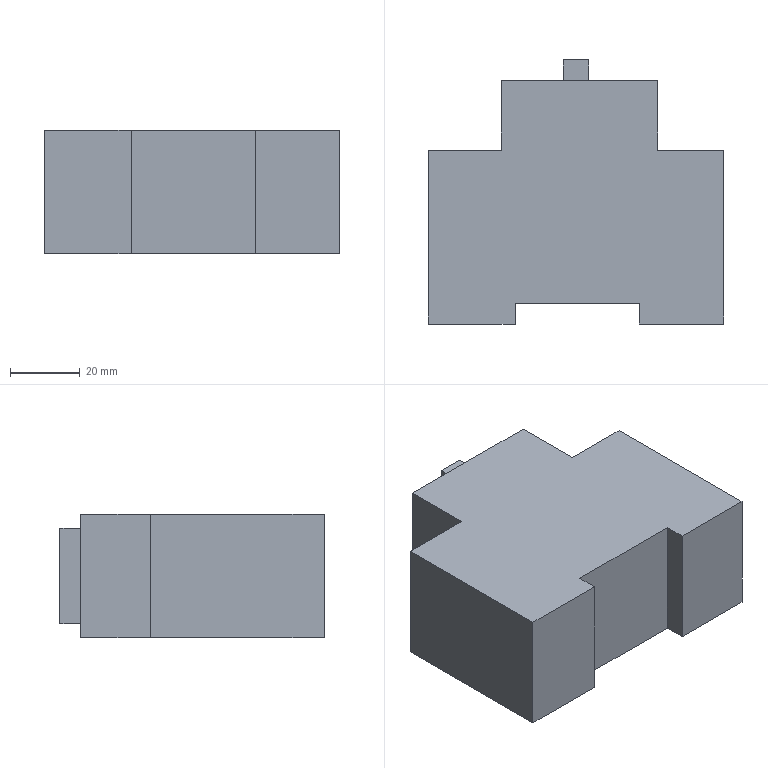Part | NX | features BREP 1 | 1 solid | 19 faces | box 85 x 76 x 35.4 mm | volume 175937 mm3 | plane 19
STEP:
#1=CARTESIAN_POINT('',(23.5,70.,-17.7));
#2=VERTEX_POINT('',#1);
#3=CARTESIAN_POINT('',(-21.5,70.,-17.7));
#4=VERTEX_POINT('',#3);
#5=CARTESIAN_POINT('',(23.5,70.,-17.7));
#6=DIRECTION('',(-1.,0.,0.));
#7=VECTOR('',#6,1000.);
#8=LINE('',#5,#7);
#9=EDGE_CURVE('',#2,#4,#8,.T.);
#10=ORIENTED_EDGE('',*,*,#9,.T.);
#11=CARTESIAN_POINT('',(-21.5,70.,17.7));
#12=VERTEX_POINT('',#11);
#13=CARTESIAN_POINT('',(-21.5,70.,17.7));
#14=DIRECTION('',(0.,0.,-1.));
#15=VECTOR('',#14,1000.);
#16=LINE('',#13,#15);
#17=EDGE_CURVE('',#12,#4,#16,.T.);
#18=ORIENTED_EDGE('',*,*,#17,.F.);
#19=CARTESIAN_POINT('',(23.5,70.,17.7));
#20=VERTEX_POINT('',#19);
#21=CARTESIAN_POINT('',(23.5,70.,17.7));
#22=DIRECTION('',(-1.,0.,0.));
#23=VECTOR('',#22,1000.);
#24=LINE('',#21,#23);
#25=EDGE_CURVE('',#20,#12,#24,.T.);
#26=ORIENTED_EDGE('',*,*,#25,.F.);
#27=CARTESIAN_POINT('',(23.5,70.,17.7));
#28=DIRECTION('',(0.,0.,-1.));
#29=VECTOR('',#28,1000.);
#30=LINE('',#27,#29);
#31=EDGE_CURVE('',#20,#2,#30,.T.);
#32=ORIENTED_EDGE('',*,*,#31,.T.);
#33=EDGE_LOOP('',(#10,#18,#26,#32));
#34=FACE_BOUND('',#33,.T.);
#35=CARTESIAN_POINT('',(3.678,70.,13.704));
#36=VERTEX_POINT('',#35);
#37=CARTESIAN_POINT('',(3.678,70.,-13.704));
#38=VERTEX_POINT('',#37);
#39=CARTESIAN_POINT('',(3.678,70.,-13.704));
#40=DIRECTION('',(0.,0.,-1.));
#41=VECTOR('',#40,1000.);
#42=LINE('',#39,#41);
#43=EDGE_CURVE('',#36,#38,#42,.T.);
#44=ORIENTED_EDGE('',*,*,#43,.F.);
#45=CARTESIAN_POINT('',(-3.678,70.,13.704));
#46=VERTEX_POINT('',#45);
#47=CARTESIAN_POINT('',(-3.678,70.,13.704));
#48=DIRECTION('',(1.,0.,0.));
#49=VECTOR('',#48,1000.);
#50=LINE('',#47,#49);
#51=EDGE_CURVE('',#46,#36,#50,.T.);
#52=ORIENTED_EDGE('',*,*,#51,.F.);
#53=CARTESIAN_POINT('',(-3.678,70.,-13.704));
#54=VERTEX_POINT('',#53);
#55=CARTESIAN_POINT('',(-3.678,70.,-13.704));
#56=DIRECTION('',(0.,0.,1.));
#57=VECTOR('',#56,1000.);
#58=LINE('',#55,#57);
#59=EDGE_CURVE('',#54,#46,#58,.T.);
#60=ORIENTED_EDGE('',*,*,#59,.F.);
#61=CARTESIAN_POINT('',(-3.678,70.,-13.704));
#62=DIRECTION('',(-1.,0.,0.));
#63=VECTOR('',#62,1000.);
#64=LINE('',#61,#63);
#65=EDGE_CURVE('',#38,#54,#64,.T.);
#66=ORIENTED_EDGE('',*,*,#65,.F.);
#67=EDGE_LOOP('',(#44,#52,#60,#66));
#68=FACE_BOUND('',#67,.T.);
#69=CARTESIAN_POINT('',(23.5,70.,17.7));
#70=DIRECTION('',(0.,-1.,0.));
#71=DIRECTION('',(1.,0.,0.));
#72=AXIS2_PLACEMENT_3D('',#69,#70,#71);
#73=PLANE('',#72);
#74=ADVANCED_FACE('',(#34,#68),#73,.F.);
#75=CARTESIAN_POINT('',(-42.5,0.,-17.7));
#76=VERTEX_POINT('',#75);
#77=CARTESIAN_POINT('',(-17.5,0.,-17.7));
#78=VERTEX_POINT('',#77);
#79=CARTESIAN_POINT('',(-42.5,0.,-17.7));
#80=DIRECTION('',(1.,0.,0.));
#81=VECTOR('',#80,1000.);
#82=LINE('',#79,#81);
#83=EDGE_CURVE('',#76,#78,#82,.T.);
#84=ORIENTED_EDGE('',*,*,#83,.T.);
#85=CARTESIAN_POINT('',(-17.5,0.,17.7));
#86=VERTEX_POINT('',#85);
#87=CARTESIAN_POINT('',(-17.5,0.,-17.7));
#88=DIRECTION('',(0.,0.,1.));
#89=VECTOR('',#88,1000.);
#90=LINE('',#87,#89);
#91=EDGE_CURVE('',#78,#86,#90,.T.);
#92=ORIENTED_EDGE('',*,*,#91,.T.);
#93=CARTESIAN_POINT('',(-42.5,0.,17.7));
#94=VERTEX_POINT('',#93);
#95=CARTESIAN_POINT('',(-42.5,0.,17.7));
#96=DIRECTION('',(1.,0.,0.));
#97=VECTOR('',#96,1000.);
#98=LINE('',#95,#97);
#99=EDGE_CURVE('',#94,#86,#98,.T.);
#100=ORIENTED_EDGE('',*,*,#99,.F.);
#101=CARTESIAN_POINT('',(-42.5,0.,17.7));
#102=DIRECTION('',(0.,0.,-1.));
#103=VECTOR('',#102,1000.);
#104=LINE('',#101,#103);
#105=EDGE_CURVE('',#94,#76,#104,.T.);
#106=ORIENTED_EDGE('',*,*,#105,.T.);
#107=EDGE_LOOP('',(#84,#92,#100,#106));
#108=FACE_BOUND('',#107,.T.);
#109=CARTESIAN_POINT('',(-42.5,0.,17.7));
#110=DIRECTION('',(0.,1.,0.));
#111=DIRECTION('',(-1.,0.,0.));
#112=AXIS2_PLACEMENT_3D('',#109,#110,#111);
#113=PLANE('',#112);
#114=ADVANCED_FACE('',(#108),#113,.F.);
#115=CARTESIAN_POINT('',(-42.5,50.,-17.7));
#116=VERTEX_POINT('',#115);
#117=CARTESIAN_POINT('',(-42.5,50.,-17.7));
#118=DIRECTION('',(0.,-1.,0.));
#119=VECTOR('',#118,1000.);
#120=LINE('',#117,#119);
#121=EDGE_CURVE('',#116,#76,#120,.T.);
#122=ORIENTED_EDGE('',*,*,#121,.T.);
#123=ORIENTED_EDGE('',*,*,#105,.F.);
#124=CARTESIAN_POINT('',(-42.5,50.,17.7));
#125=VERTEX_POINT('',#124);
#126=CARTESIAN_POINT('',(-42.5,50.,17.7));
#127=DIRECTION('',(0.,-1.,0.));
#128=VECTOR('',#127,1000.);
#129=LINE('',#126,#128);
#130=EDGE_CURVE('',#125,#94,#129,.T.);
#131=ORIENTED_EDGE('',*,*,#130,.F.);
#132=CARTESIAN_POINT('',(-42.5,50.,17.7));
#133=DIRECTION('',(0.,0.,-1.));
#134=VECTOR('',#133,1000.);
#135=LINE('',#132,#134);
#136=EDGE_CURVE('',#125,#116,#135,.T.);
#137=ORIENTED_EDGE('',*,*,#136,.T.);
#138=EDGE_LOOP('',(#122,#123,#131,#137));
#139=FACE_BOUND('',#138,.T.);
#140=CARTESIAN_POINT('',(-42.5,50.,17.7));
#141=DIRECTION('',(1.,0.,0.));
#142=DIRECTION('',(0.,1.,0.));
#143=AXIS2_PLACEMENT_3D('',#140,#141,#142);
#144=PLANE('',#143);
#145=ADVANCED_FACE('',(#139),#144,.F.);
#146=CARTESIAN_POINT('',(18.2,0.,17.7));
#147=VERTEX_POINT('',#146);
#148=CARTESIAN_POINT('',(42.5,0.,17.7));
#149=VERTEX_POINT('',#148);
#150=CARTESIAN_POINT('',(-42.5,0.,17.7));
#151=DIRECTION('',(1.,0.,0.));
#152=VECTOR('',#151,1000.);
#153=LINE('',#150,#152);
#154=EDGE_CURVE('',#147,#149,#153,.T.);
#155=ORIENTED_EDGE('',*,*,#154,.F.);
#156=CARTESIAN_POINT('',(18.2,0.,-17.7));
#157=VERTEX_POINT('',#156);
#158=CARTESIAN_POINT('',(18.2,0.,-17.7));
#159=DIRECTION('',(0.,0.,1.));
#160=VECTOR('',#159,1000.);
#161=LINE('',#158,#160);
#162=EDGE_CURVE('',#157,#147,#161,.T.);
#163=ORIENTED_EDGE('',*,*,#162,.F.);
#164=CARTESIAN_POINT('',(42.5,0.,-17.7));
#165=VERTEX_POINT('',#164);
#166=CARTESIAN_POINT('',(-42.5,0.,-17.7));
#167=DIRECTION('',(1.,0.,0.));
#168=VECTOR('',#167,1000.);
#169=LINE('',#166,#168);
#170=EDGE_CURVE('',#157,#165,#169,.T.);
#171=ORIENTED_EDGE('',*,*,#170,.T.);
#172=CARTESIAN_POINT('',(42.5,0.,17.7));
#173=DIRECTION('',(0.,0.,-1.));
#174=VECTOR('',#173,1000.);
#175=LINE('',#172,#174);
#176=EDGE_CURVE('',#149,#165,#175,.T.);
#177=ORIENTED_EDGE('',*,*,#176,.F.);
#178=EDGE_LOOP('',(#155,#163,#171,#177));
#179=FACE_BOUND('',#178,.T.);
#180=CARTESIAN_POINT('',(-42.5,0.,17.7));
#181=DIRECTION('',(0.,1.,0.));
#182=DIRECTION('',(-1.,0.,0.));
#183=AXIS2_PLACEMENT_3D('',#180,#181,#182);
#184=PLANE('',#183);
#185=ADVANCED_FACE('',(#179),#184,.F.);
#186=CARTESIAN_POINT('',(42.5,50.,-17.7));
#187=VERTEX_POINT('',#186);
#188=CARTESIAN_POINT('',(42.5,0.,-17.7));
#189=DIRECTION('',(0.,1.,0.));
#190=VECTOR('',#189,1000.);
#191=LINE('',#188,#190);
#192=EDGE_CURVE('',#165,#187,#191,.T.);
#193=ORIENTED_EDGE('',*,*,#192,.T.);
#194=CARTESIAN_POINT('',(42.5,50.,17.7));
#195=VERTEX_POINT('',#194);
#196=CARTESIAN_POINT('',(42.5,50.,17.7));
#197=DIRECTION('',(0.,0.,-1.));
#198=VECTOR('',#197,1000.);
#199=LINE('',#196,#198);
#200=EDGE_CURVE('',#195,#187,#199,.T.);
#201=ORIENTED_EDGE('',*,*,#200,.F.);
#202=CARTESIAN_POINT('',(42.5,0.,17.7));
#203=DIRECTION('',(0.,1.,0.));
#204=VECTOR('',#203,1000.);
#205=LINE('',#202,#204);
#206=EDGE_CURVE('',#149,#195,#205,.T.);
#207=ORIENTED_EDGE('',*,*,#206,.F.);
#208=ORIENTED_EDGE('',*,*,#176,.T.);
#209=EDGE_LOOP('',(#193,#201,#207,#208));
#210=FACE_BOUND('',#209,.T.);
#211=CARTESIAN_POINT('',(42.5,0.,17.7));
#212=DIRECTION('',(-1.,0.,0.));
#213=DIRECTION('',(0.,0.,1.));
#214=AXIS2_PLACEMENT_3D('',#211,#212,#213);
#215=PLANE('',#214);
#216=ADVANCED_FACE('',(#210),#215,.F.);
#217=CARTESIAN_POINT('',(23.5,50.,-17.7));
#218=VERTEX_POINT('',#217);
#219=CARTESIAN_POINT('',(42.5,50.,-17.7));
#220=DIRECTION('',(-1.,0.,0.));
#221=VECTOR('',#220,1000.);
#222=LINE('',#219,#221);
#223=EDGE_CURVE('',#187,#218,#222,.T.);
#224=ORIENTED_EDGE('',*,*,#223,.T.);
#225=CARTESIAN_POINT('',(23.5,50.,17.7));
#226=VERTEX_POINT('',#225);
#227=CARTESIAN_POINT('',(23.5,50.,17.7));
#228=DIRECTION('',(0.,0.,-1.));
#229=VECTOR('',#228,1000.);
#230=LINE('',#227,#229);
#231=EDGE_CURVE('',#226,#218,#230,.T.);
#232=ORIENTED_EDGE('',*,*,#231,.F.);
#233=CARTESIAN_POINT('',(42.5,50.,17.7));
#234=DIRECTION('',(-1.,0.,0.));
#235=VECTOR('',#234,1000.);
#236=LINE('',#233,#235);
#237=EDGE_CURVE('',#195,#226,#236,.T.);
#238=ORIENTED_EDGE('',*,*,#237,.F.);
#239=ORIENTED_EDGE('',*,*,#200,.T.);
#240=EDGE_LOOP('',(#224,#232,#238,#239));
#241=FACE_BOUND('',#240,.T.);
#242=CARTESIAN_POINT('',(42.5,50.,17.7));
#243=DIRECTION('',(0.,-1.,0.));
#244=DIRECTION('',(0.,0.,-1.));
#245=AXIS2_PLACEMENT_3D('',#242,#243,#244);
#246=PLANE('',#245);
#247=ADVANCED_FACE('',(#241),#246,.F.);
#248=CARTESIAN_POINT('',(23.5,50.,-17.7));
#249=DIRECTION('',(0.,1.,0.));
#250=VECTOR('',#249,1000.);
#251=LINE('',#248,#250);
#252=EDGE_CURVE('',#218,#2,#251,.T.);
#253=ORIENTED_EDGE('',*,*,#252,.T.);
#254=ORIENTED_EDGE('',*,*,#31,.F.);
#255=CARTESIAN_POINT('',(23.5,50.,17.7));
#256=DIRECTION('',(0.,1.,0.));
#257=VECTOR('',#256,1000.);
#258=LINE('',#255,#257);
#259=EDGE_CURVE('',#226,#20,#258,.T.);
#260=ORIENTED_EDGE('',*,*,#259,.F.);
#261=ORIENTED_EDGE('',*,*,#231,.T.);
#262=EDGE_LOOP('',(#253,#254,#260,#261));
#263=FACE_BOUND('',#262,.T.);
#264=CARTESIAN_POINT('',(23.5,50.,17.7));
#265=DIRECTION('',(-1.,0.,0.));
#266=DIRECTION('',(0.,0.,1.));
#267=AXIS2_PLACEMENT_3D('',#264,#265,#266);
#268=PLANE('',#267);
#269=ADVANCED_FACE('',(#263),#268,.F.);
#270=CARTESIAN_POINT('',(-21.5,50.,-17.7));
#271=VERTEX_POINT('',#270);
#272=CARTESIAN_POINT('',(-21.5,70.,-17.7));
#273=DIRECTION('',(0.,-1.,0.));
#274=VECTOR('',#273,1000.);
#275=LINE('',#272,#274);
#276=EDGE_CURVE('',#4,#271,#275,.T.);
#277=ORIENTED_EDGE('',*,*,#276,.T.);
#278=CARTESIAN_POINT('',(-21.5,50.,17.7));
#279=VERTEX_POINT('',#278);
#280=CARTESIAN_POINT('',(-21.5,50.,17.7));
#281=DIRECTION('',(0.,0.,-1.));
#282=VECTOR('',#281,1000.);
#283=LINE('',#280,#282);
#284=EDGE_CURVE('',#279,#271,#283,.T.);
#285=ORIENTED_EDGE('',*,*,#284,.F.);
#286=CARTESIAN_POINT('',(-21.5,70.,17.7));
#287=DIRECTION('',(0.,-1.,0.));
#288=VECTOR('',#287,1000.);
#289=LINE('',#286,#288);
#290=EDGE_CURVE('',#12,#279,#289,.T.);
#291=ORIENTED_EDGE('',*,*,#290,.F.);
#292=ORIENTED_EDGE('',*,*,#17,.T.);
#293=EDGE_LOOP('',(#277,#285,#291,#292));
#294=FACE_BOUND('',#293,.T.);
#295=CARTESIAN_POINT('',(-21.5,70.,17.7));
#296=DIRECTION('',(1.,0.,0.));
#297=DIRECTION('',(0.,1.,0.));
#298=AXIS2_PLACEMENT_3D('',#295,#296,#297);
#299=PLANE('',#298);
#300=ADVANCED_FACE('',(#294),#299,.F.);
#301=CARTESIAN_POINT('',(-21.5,50.,-17.7));
#302=DIRECTION('',(-1.,0.,0.));
#303=VECTOR('',#302,1000.);
#304=LINE('',#301,#303);
#305=EDGE_CURVE('',#271,#116,#304,.T.);
#306=ORIENTED_EDGE('',*,*,#305,.T.);
#307=ORIENTED_EDGE('',*,*,#136,.F.);
#308=CARTESIAN_POINT('',(-21.5,50.,17.7));
#309=DIRECTION('',(-1.,0.,0.));
#310=VECTOR('',#309,1000.);
#311=LINE('',#308,#310);
#312=EDGE_CURVE('',#279,#125,#311,.T.);
#313=ORIENTED_EDGE('',*,*,#312,.F.);
#314=ORIENTED_EDGE('',*,*,#284,.T.);
#315=EDGE_LOOP('',(#306,#307,#313,#314));
#316=FACE_BOUND('',#315,.T.);
#317=CARTESIAN_POINT('',(-21.5,50.,17.7));
#318=DIRECTION('',(0.,-1.,0.));
#319=DIRECTION('',(1.,0.,0.));
#320=AXIS2_PLACEMENT_3D('',#317,#318,#319);
#321=PLANE('',#320);
#322=ADVANCED_FACE('',(#316),#321,.F.);
#323=CARTESIAN_POINT('',(-17.5,6.,17.7));
#324=VERTEX_POINT('',#323);
#325=CARTESIAN_POINT('',(-17.5,0.,17.7));
#326=DIRECTION('',(0.,-1.,0.));
#327=VECTOR('',#326,1000.);
#328=LINE('',#325,#327);
#329=EDGE_CURVE('',#324,#86,#328,.T.);
#330=ORIENTED_EDGE('',*,*,#329,.F.);
#331=CARTESIAN_POINT('',(18.2,6.,17.7));
#332=VERTEX_POINT('',#331);
#333=CARTESIAN_POINT('',(-17.5,6.,17.7));
#334=DIRECTION('',(-1.,0.,0.));
#335=VECTOR('',#334,1000.);
#336=LINE('',#333,#335);
#337=EDGE_CURVE('',#332,#324,#336,.T.);
#338=ORIENTED_EDGE('',*,*,#337,.F.);
#339=CARTESIAN_POINT('',(18.2,0.,17.7));
#340=DIRECTION('',(0.,1.,0.));
#341=VECTOR('',#340,1000.);
#342=LINE('',#339,#341);
#343=EDGE_CURVE('',#147,#332,#342,.T.);
#344=ORIENTED_EDGE('',*,*,#343,.F.);
#345=ORIENTED_EDGE('',*,*,#154,.T.);
#346=ORIENTED_EDGE('',*,*,#206,.T.);
#347=ORIENTED_EDGE('',*,*,#237,.T.);
#348=ORIENTED_EDGE('',*,*,#259,.T.);
#349=ORIENTED_EDGE('',*,*,#25,.T.);
#350=ORIENTED_EDGE('',*,*,#290,.T.);
#351=ORIENTED_EDGE('',*,*,#312,.T.);
#352=ORIENTED_EDGE('',*,*,#130,.T.);
#353=ORIENTED_EDGE('',*,*,#99,.T.);
#354=EDGE_LOOP('',(#330,#338,#344,#345,#346,#347,#348,#349,#350,#351,#352,#353));
#355=FACE_BOUND('',#354,.T.);
#356=CARTESIAN_POINT('',(0.,0.,17.7));
#357=DIRECTION('',(0.,0.,1.));
#358=DIRECTION('',(1.,0.,0.));
#359=AXIS2_PLACEMENT_3D('',#356,#357,#358);
#360=PLANE('',#359);
#361=ADVANCED_FACE('',(#355),#360,.T.);
#362=CARTESIAN_POINT('',(18.2,6.,-17.7));
#363=VERTEX_POINT('',#362);
#364=CARTESIAN_POINT('',(-17.5,6.,-17.7));
#365=VERTEX_POINT('',#364);
#366=CARTESIAN_POINT('',(-17.5,6.,-17.7));
#367=DIRECTION('',(-1.,0.,0.));
#368=VECTOR('',#367,1000.);
#369=LINE('',#366,#368);
#370=EDGE_CURVE('',#363,#365,#369,.T.);
#371=ORIENTED_EDGE('',*,*,#370,.T.);
#372=CARTESIAN_POINT('',(-17.5,0.,-17.7));
#373=DIRECTION('',(0.,-1.,0.));
#374=VECTOR('',#373,1000.);
#375=LINE('',#372,#374);
#376=EDGE_CURVE('',#365,#78,#375,.T.);
#377=ORIENTED_EDGE('',*,*,#376,.T.);
#378=ORIENTED_EDGE('',*,*,#83,.F.);
#379=ORIENTED_EDGE('',*,*,#121,.F.);
#380=ORIENTED_EDGE('',*,*,#305,.F.);
#381=ORIENTED_EDGE('',*,*,#276,.F.);
#382=ORIENTED_EDGE('',*,*,#9,.F.);
#383=ORIENTED_EDGE('',*,*,#252,.F.);
#384=ORIENTED_EDGE('',*,*,#223,.F.);
#385=ORIENTED_EDGE('',*,*,#192,.F.);
#386=ORIENTED_EDGE('',*,*,#170,.F.);
#387=CARTESIAN_POINT('',(18.2,0.,-17.7));
#388=DIRECTION('',(0.,1.,0.));
#389=VECTOR('',#388,1000.);
#390=LINE('',#387,#389);
#391=EDGE_CURVE('',#157,#363,#390,.T.);
#392=ORIENTED_EDGE('',*,*,#391,.T.);
#393=EDGE_LOOP('',(#371,#377,#378,#379,#380,#381,#382,#383,#384,#385,#386,#392));
#394=FACE_BOUND('',#393,.T.);
#395=CARTESIAN_POINT('',(0.,0.,-17.7));
#396=DIRECTION('',(0.,0.,1.));
#397=DIRECTION('',(1.,0.,0.));
#398=AXIS2_PLACEMENT_3D('',#395,#396,#397);
#399=PLANE('',#398);
#400=ADVANCED_FACE('',(#394),#399,.F.);
#401=ORIENTED_EDGE('',*,*,#329,.T.);
#402=ORIENTED_EDGE('',*,*,#91,.F.);
#403=ORIENTED_EDGE('',*,*,#376,.F.);
#404=CARTESIAN_POINT('',(-17.5,6.,-17.7));
#405=DIRECTION('',(0.,0.,1.));
#406=VECTOR('',#405,1000.);
#407=LINE('',#404,#406);
#408=EDGE_CURVE('',#365,#324,#407,.T.);
#409=ORIENTED_EDGE('',*,*,#408,.T.);
#410=EDGE_LOOP('',(#401,#402,#403,#409));
#411=FACE_BOUND('',#410,.T.);
#412=CARTESIAN_POINT('',(-17.5,0.,-17.7));
#413=DIRECTION('',(-1.,0.,0.));
#414=DIRECTION('',(0.,0.,1.));
#415=AXIS2_PLACEMENT_3D('',#412,#413,#414);
#416=PLANE('',#415);
#417=ADVANCED_FACE('',(#411),#416,.F.);
#418=ORIENTED_EDGE('',*,*,#337,.T.);
#419=ORIENTED_EDGE('',*,*,#408,.F.);
#420=ORIENTED_EDGE('',*,*,#370,.F.);
#421=CARTESIAN_POINT('',(18.2,6.,-17.7));
#422=DIRECTION('',(0.,0.,1.));
#423=VECTOR('',#422,1000.);
#424=LINE('',#421,#423);
#425=EDGE_CURVE('',#363,#332,#424,.T.);
#426=ORIENTED_EDGE('',*,*,#425,.T.);
#427=EDGE_LOOP('',(#418,#419,#420,#426));
#428=FACE_BOUND('',#427,.T.);
#429=CARTESIAN_POINT('',(-17.5,6.,-17.7));
#430=DIRECTION('',(0.,1.,0.));
#431=DIRECTION('',(0.,0.,1.));
#432=AXIS2_PLACEMENT_3D('',#429,#430,#431);
#433=PLANE('',#432);
#434=ADVANCED_FACE('',(#428),#433,.F.);
#435=ORIENTED_EDGE('',*,*,#343,.T.);
#436=ORIENTED_EDGE('',*,*,#425,.F.);
#437=ORIENTED_EDGE('',*,*,#391,.F.);
#438=ORIENTED_EDGE('',*,*,#162,.T.);
#439=EDGE_LOOP('',(#435,#436,#437,#438));
#440=FACE_BOUND('',#439,.T.);
#441=CARTESIAN_POINT('',(18.2,0.,-17.7));
#442=DIRECTION('',(1.,0.,0.));
#443=DIRECTION('',(0.,0.,-1.));
#444=AXIS2_PLACEMENT_3D('',#441,#442,#443);
#445=PLANE('',#444);
#446=ADVANCED_FACE('',(#440),#445,.F.);
#447=ORIENTED_EDGE('',*,*,#43,.T.);
#448=CARTESIAN_POINT('',(3.678,76.,-13.704));
#449=VERTEX_POINT('',#448);
#450=CARTESIAN_POINT('',(3.678,76.,-13.704));
#451=DIRECTION('',(0.,-1.,0.));
#452=VECTOR('',#451,1000.);
#453=LINE('',#450,#452);
#454=EDGE_CURVE('',#449,#38,#453,.T.);
#455=ORIENTED_EDGE('',*,*,#454,.F.);
#456=CARTESIAN_POINT('',(3.678,76.,13.704));
#457=VERTEX_POINT('',#456);
#458=CARTESIAN_POINT('',(3.678,76.,-13.704));
#459=DIRECTION('',(0.,0.,-1.));
#460=VECTOR('',#459,1000.);
#461=LINE('',#458,#460);
#462=EDGE_CURVE('',#457,#449,#461,.T.);
#463=ORIENTED_EDGE('',*,*,#462,.F.);
#464=CARTESIAN_POINT('',(3.678,76.,13.704));
#465=DIRECTION('',(0.,-1.,0.));
#466=VECTOR('',#465,1000.);
#467=LINE('',#464,#466);
#468=EDGE_CURVE('',#457,#36,#467,.T.);
#469=ORIENTED_EDGE('',*,*,#468,.T.);
#470=EDGE_LOOP('',(#447,#455,#463,#469));
#471=FACE_BOUND('',#470,.T.);
#472=CARTESIAN_POINT('',(3.678,76.,-13.704));
#473=DIRECTION('',(-1.,0.,0.));
#474=DIRECTION('',(0.,-1.,0.));
#475=AXIS2_PLACEMENT_3D('',#472,#473,#474);
#476=PLANE('',#475);
#477=ADVANCED_FACE('',(#471),#476,.F.);
#478=ORIENTED_EDGE('',*,*,#65,.T.);
#479=CARTESIAN_POINT('',(-3.678,76.,-13.704));
#480=VERTEX_POINT('',#479);
#481=CARTESIAN_POINT('',(-3.678,76.,-13.704));
#482=DIRECTION('',(0.,-1.,0.));
#483=VECTOR('',#482,1000.);
#484=LINE('',#481,#483);
#485=EDGE_CURVE('',#480,#54,#484,.T.);
#486=ORIENTED_EDGE('',*,*,#485,.F.);
#487=CARTESIAN_POINT('',(-3.678,76.,-13.704));
#488=DIRECTION('',(-1.,0.,0.));
#489=VECTOR('',#488,1000.);
#490=LINE('',#487,#489);
#491=EDGE_CURVE('',#449,#480,#490,.T.);
#492=ORIENTED_EDGE('',*,*,#491,.F.);
#493=ORIENTED_EDGE('',*,*,#454,.T.);
#494=EDGE_LOOP('',(#478,#486,#492,#493));
#495=FACE_BOUND('',#494,.T.);
#496=CARTESIAN_POINT('',(-3.678,76.,-13.704));
#497=DIRECTION('',(0.,0.,1.));
#498=DIRECTION('',(1.,0.,0.));
#499=AXIS2_PLACEMENT_3D('',#496,#497,#498);
#500=PLANE('',#499);
#501=ADVANCED_FACE('',(#495),#500,.F.);
#502=ORIENTED_EDGE('',*,*,#59,.T.);
#503=CARTESIAN_POINT('',(-3.678,76.,13.704));
#504=VERTEX_POINT('',#503);
#505=CARTESIAN_POINT('',(-3.678,76.,13.704));
#506=DIRECTION('',(0.,-1.,0.));
#507=VECTOR('',#506,1000.);
#508=LINE('',#505,#507);
#509=EDGE_CURVE('',#504,#46,#508,.T.);
#510=ORIENTED_EDGE('',*,*,#509,.F.);
#511=CARTESIAN_POINT('',(-3.678,76.,-13.704));
#512=DIRECTION('',(0.,0.,1.));
#513=VECTOR('',#512,1000.);
#514=LINE('',#511,#513);
#515=EDGE_CURVE('',#480,#504,#514,.T.);
#516=ORIENTED_EDGE('',*,*,#515,.F.);
#517=ORIENTED_EDGE('',*,*,#485,.T.);
#518=EDGE_LOOP('',(#502,#510,#516,#517));
#519=FACE_BOUND('',#518,.T.);
#520=CARTESIAN_POINT('',(-3.678,76.,-13.704));
#521=DIRECTION('',(1.,0.,0.));
#522=DIRECTION('',(0.,1.,0.));
#523=AXIS2_PLACEMENT_3D('',#520,#521,#522);
#524=PLANE('',#523);
#525=ADVANCED_FACE('',(#519),#524,.F.);
#526=ORIENTED_EDGE('',*,*,#51,.T.);
#527=ORIENTED_EDGE('',*,*,#468,.F.);
#528=CARTESIAN_POINT('',(-3.678,76.,13.704));
#529=DIRECTION('',(1.,0.,0.));
#530=VECTOR('',#529,1000.);
#531=LINE('',#528,#530);
#532=EDGE_CURVE('',#504,#457,#531,.T.);
#533=ORIENTED_EDGE('',*,*,#532,.F.);
#534=ORIENTED_EDGE('',*,*,#509,.T.);
#535=EDGE_LOOP('',(#526,#527,#533,#534));
#536=FACE_BOUND('',#535,.T.);
#537=CARTESIAN_POINT('',(-3.678,76.,13.704));
#538=DIRECTION('',(0.,0.,-1.));
#539=DIRECTION('',(-1.,0.,0.));
#540=AXIS2_PLACEMENT_3D('',#537,#538,#539);
#541=PLANE('',#540);
#542=ADVANCED_FACE('',(#536),#541,.F.);
#543=ORIENTED_EDGE('',*,*,#462,.T.);
#544=ORIENTED_EDGE('',*,*,#491,.T.);
#545=ORIENTED_EDGE('',*,*,#515,.T.);
#546=ORIENTED_EDGE('',*,*,#532,.T.);
#547=EDGE_LOOP('',(#543,#544,#545,#546));
#548=FACE_BOUND('',#547,.T.);
#549=CARTESIAN_POINT('',(0.,76.,0.));
#550=DIRECTION('',(0.,1.,0.));
#551=DIRECTION('',(0.,0.,1.));
#552=AXIS2_PLACEMENT_3D('',#549,#550,#551);
#553=PLANE('',#552);
#554=ADVANCED_FACE('',(#548),#553,.T.);
#555=CLOSED_SHELL('',(#74,#114,#145,#185,#216,#247,#269,#300,#322,#361,#400,#417,#434,#446,#477,#501,#525,#542,#554));
#556=MANIFOLD_SOLID_BREP('',#555);
#557=(LENGTH_UNIT()NAMED_UNIT(*)SI_UNIT(.MILLI.,.METRE.));
#558=UNCERTAINTY_MEASURE_WITH_UNIT(LENGTH_MEASURE(0.00001),#557,'','');
#559=(NAMED_UNIT(*)PLANE_ANGLE_UNIT()SI_UNIT($,.RADIAN.));
#560=(NAMED_UNIT(*)SI_UNIT($,.STERADIAN.)SOLID_ANGLE_UNIT());
#561=(GEOMETRIC_REPRESENTATION_CONTEXT(3)GLOBAL_UNCERTAINTY_ASSIGNED_CONTEXT((#558))GLOBAL_UNIT_ASSIGNED_CONTEXT((#557,#559,#560))REPRESENTATION_CONTEXT('',''));
#562=ADVANCED_BREP_SHAPE_REPRESENTATION('',(#556),#561);